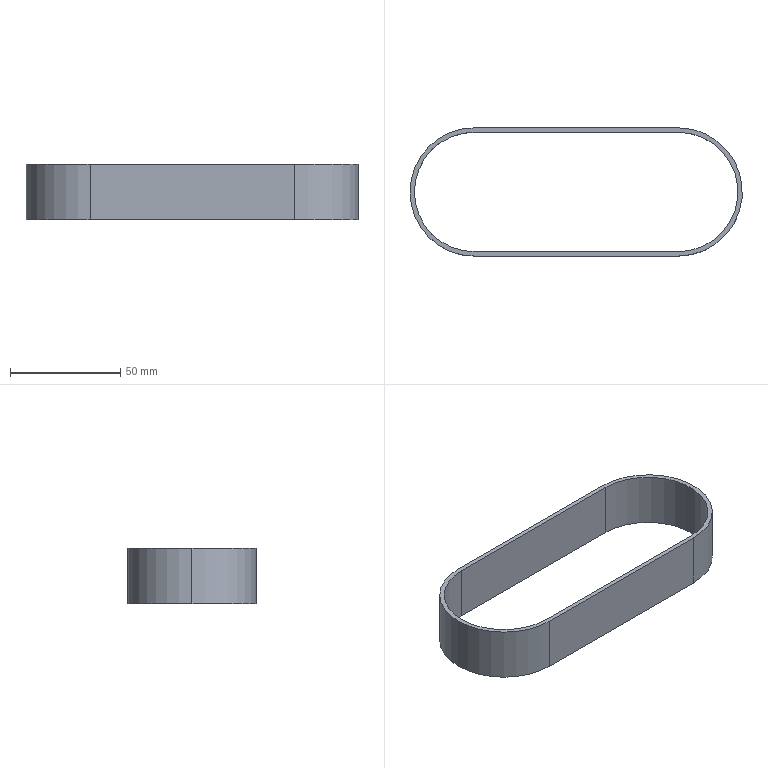Part | STEP file | HTBNV355-S5M-250 high-torque timing belt S5M MISUMI 24 | 1 solid | 12 faces | box 150.61 x 58.11 x 25 mm | volume 18064 mm3 | cylinder 6 | plane 6 | commonest cylinder face diameters 54.11 x3 58.11 x3
STEP:
#1=CARTESIAN_POINT('',(-46.25,27.055,12.5));
#2=VERTEX_POINT('',#1);
#3=CARTESIAN_POINT('',(-73.305,0.,12.5));
#4=VERTEX_POINT('',#3);
#5=CARTESIAN_POINT('',(-46.25,0.,12.5));
#6=DIRECTION('',(0.,0.,1.));
#7=DIRECTION('',(1.,0.,0.));
#8=AXIS2_PLACEMENT_3D('',#5,#6,#7);
#9=CIRCLE('',#8,27.055);
#10=EDGE_CURVE('',#2,#4,#9,.T.);
#11=ORIENTED_EDGE('',*,*,#10,.T.);
#12=CARTESIAN_POINT('',(-73.305,0.,-12.5));
#13=VERTEX_POINT('',#12);
#14=CARTESIAN_POINT('',(-73.305,0.,12.5));
#15=DIRECTION('',(0.,0.,-1.));
#16=VECTOR('',#15,1000.);
#17=LINE('',#14,#16);
#18=EDGE_CURVE('',#4,#13,#17,.T.);
#19=ORIENTED_EDGE('',*,*,#18,.T.);
#20=CARTESIAN_POINT('',(-46.25,27.055,-12.5));
#21=VERTEX_POINT('',#20);
#22=CARTESIAN_POINT('',(-46.25,0.,-12.5));
#23=DIRECTION('',(0.,0.,1.));
#24=DIRECTION('',(1.,0.,0.));
#25=AXIS2_PLACEMENT_3D('',#22,#23,#24);
#26=CIRCLE('',#25,27.055);
#27=EDGE_CURVE('',#21,#13,#26,.T.);
#28=ORIENTED_EDGE('',*,*,#27,.F.);
#29=CARTESIAN_POINT('',(-46.25,27.055,12.5));
#30=DIRECTION('',(0.,0.,-1.));
#31=VECTOR('',#30,1000.);
#32=LINE('',#29,#31);
#33=EDGE_CURVE('',#2,#21,#32,.T.);
#34=ORIENTED_EDGE('',*,*,#33,.F.);
#35=EDGE_LOOP('',(#11,#19,#28,#34));
#36=FACE_OUTER_BOUND('',#35,.T.);
#37=CARTESIAN_POINT('',(-46.25,0.,12.5));
#38=DIRECTION('',(0.,0.,-1.));
#39=DIRECTION('',(-1.,0.,0.));
#40=AXIS2_PLACEMENT_3D('',#37,#38,#39);
#41=CYLINDRICAL_SURFACE('',#40,27.055);
#42=ADVANCED_FACE('',(#36),#41,.F.);
#43=CARTESIAN_POINT('',(-75.305,0.,12.5));
#44=VERTEX_POINT('',#43);
#45=CARTESIAN_POINT('',(-46.25,-29.055,12.5));
#46=VERTEX_POINT('',#45);
#47=CARTESIAN_POINT('',(-46.25,0.,12.5));
#48=DIRECTION('',(0.,0.,1.));
#49=DIRECTION('',(1.,0.,0.));
#50=AXIS2_PLACEMENT_3D('',#47,#48,#49);
#51=CIRCLE('',#50,29.055);
#52=EDGE_CURVE('',#44,#46,#51,.T.);
#53=ORIENTED_EDGE('',*,*,#52,.F.);
#54=CARTESIAN_POINT('',(-75.305,0.,-12.5));
#55=VERTEX_POINT('',#54);
#56=CARTESIAN_POINT('',(-75.305,0.,12.5));
#57=DIRECTION('',(0.,0.,-1.));
#58=VECTOR('',#57,1000.);
#59=LINE('',#56,#58);
#60=EDGE_CURVE('',#44,#55,#59,.T.);
#61=ORIENTED_EDGE('',*,*,#60,.T.);
#62=CARTESIAN_POINT('',(-46.25,-29.055,-12.5));
#63=VERTEX_POINT('',#62);
#64=CARTESIAN_POINT('',(-46.25,0.,-12.5));
#65=DIRECTION('',(0.,0.,1.));
#66=DIRECTION('',(1.,0.,0.));
#67=AXIS2_PLACEMENT_3D('',#64,#65,#66);
#68=CIRCLE('',#67,29.055);
#69=EDGE_CURVE('',#55,#63,#68,.T.);
#70=ORIENTED_EDGE('',*,*,#69,.T.);
#71=CARTESIAN_POINT('',(-46.25,-29.055,12.5));
#72=DIRECTION('',(0.,0.,-1.));
#73=VECTOR('',#72,1000.);
#74=LINE('',#71,#73);
#75=EDGE_CURVE('',#46,#63,#74,.T.);
#76=ORIENTED_EDGE('',*,*,#75,.F.);
#77=EDGE_LOOP('',(#53,#61,#70,#76));
#78=FACE_OUTER_BOUND('',#77,.T.);
#79=CARTESIAN_POINT('',(-46.25,0.,12.5));
#80=DIRECTION('',(0.,0.,-1.));
#81=DIRECTION('',(-1.,0.,0.));
#82=AXIS2_PLACEMENT_3D('',#79,#80,#81);
#83=CYLINDRICAL_SURFACE('',#82,29.055);
#84=ADVANCED_FACE('',(#78),#83,.T.);
#85=CARTESIAN_POINT('',(-46.25,29.055,12.5));
#86=VERTEX_POINT('',#85);
#87=CARTESIAN_POINT('',(-46.25,0.,12.5));
#88=DIRECTION('',(0.,0.,1.));
#89=DIRECTION('',(1.,0.,0.));
#90=AXIS2_PLACEMENT_3D('',#87,#88,#89);
#91=CIRCLE('',#90,29.055);
#92=EDGE_CURVE('',#86,#44,#91,.T.);
#93=ORIENTED_EDGE('',*,*,#92,.T.);
#94=ORIENTED_EDGE('',*,*,#52,.T.);
#95=CARTESIAN_POINT('',(46.25,-29.055,12.5));
#96=VERTEX_POINT('',#95);
#97=CARTESIAN_POINT('',(-46.25,-29.055,12.5));
#98=DIRECTION('',(1.,0.,0.));
#99=VECTOR('',#98,1000.);
#100=LINE('',#97,#99);
#101=EDGE_CURVE('',#46,#96,#100,.T.);
#102=ORIENTED_EDGE('',*,*,#101,.T.);
#103=CARTESIAN_POINT('',(46.25,29.055,12.5));
#104=VERTEX_POINT('',#103);
#105=CARTESIAN_POINT('',(46.25,0.,12.5));
#106=DIRECTION('',(0.,0.,1.));
#107=DIRECTION('',(1.,0.,0.));
#108=AXIS2_PLACEMENT_3D('',#105,#106,#107);
#109=CIRCLE('',#108,29.055);
#110=EDGE_CURVE('',#96,#104,#109,.T.);
#111=ORIENTED_EDGE('',*,*,#110,.T.);
#112=CARTESIAN_POINT('',(-46.25,29.055,12.5));
#113=DIRECTION('',(-1.,0.,0.));
#114=VECTOR('',#113,1000.);
#115=LINE('',#112,#114);
#116=EDGE_CURVE('',#104,#86,#115,.T.);
#117=ORIENTED_EDGE('',*,*,#116,.T.);
#118=EDGE_LOOP('',(#93,#94,#102,#111,#117));
#119=FACE_OUTER_BOUND('',#118,.T.);
#120=CARTESIAN_POINT('',(-46.25,-27.055,12.5));
#121=VERTEX_POINT('',#120);
#122=CARTESIAN_POINT('',(46.25,-27.055,12.5));
#123=VERTEX_POINT('',#122);
#124=CARTESIAN_POINT('',(-46.25,-27.055,12.5));
#125=DIRECTION('',(1.,0.,0.));
#126=VECTOR('',#125,1000.);
#127=LINE('',#124,#126);
#128=EDGE_CURVE('',#121,#123,#127,.T.);
#129=ORIENTED_EDGE('',*,*,#128,.F.);
#130=CARTESIAN_POINT('',(-46.25,0.,12.5));
#131=DIRECTION('',(0.,0.,1.));
#132=DIRECTION('',(1.,0.,0.));
#133=AXIS2_PLACEMENT_3D('',#130,#131,#132);
#134=CIRCLE('',#133,27.055);
#135=EDGE_CURVE('',#4,#121,#134,.T.);
#136=ORIENTED_EDGE('',*,*,#135,.F.);
#137=ORIENTED_EDGE('',*,*,#10,.F.);
#138=CARTESIAN_POINT('',(46.25,27.055,12.5));
#139=VERTEX_POINT('',#138);
#140=CARTESIAN_POINT('',(-46.25,27.055,12.5));
#141=DIRECTION('',(-1.,0.,0.));
#142=VECTOR('',#141,1000.);
#143=LINE('',#140,#142);
#144=EDGE_CURVE('',#139,#2,#143,.T.);
#145=ORIENTED_EDGE('',*,*,#144,.F.);
#146=CARTESIAN_POINT('',(46.25,0.,12.5));
#147=DIRECTION('',(0.,0.,1.));
#148=DIRECTION('',(1.,0.,0.));
#149=AXIS2_PLACEMENT_3D('',#146,#147,#148);
#150=CIRCLE('',#149,27.055);
#151=EDGE_CURVE('',#123,#139,#150,.T.);
#152=ORIENTED_EDGE('',*,*,#151,.F.);
#153=EDGE_LOOP('',(#129,#136,#137,#145,#152));
#154=FACE_BOUND('',#153,.T.);
#155=CARTESIAN_POINT('',(-46.25,0.,12.5));
#156=DIRECTION('',(0.,0.,1.));
#157=DIRECTION('',(1.,0.,0.));
#158=AXIS2_PLACEMENT_3D('',#155,#156,#157);
#159=PLANE('',#158);
#160=ADVANCED_FACE('',(#119,#154),#159,.T.);
#161=CARTESIAN_POINT('',(-46.25,29.055,-12.5));
#162=VERTEX_POINT('',#161);
#163=CARTESIAN_POINT('',(-46.25,0.,-12.5));
#164=DIRECTION('',(0.,0.,1.));
#165=DIRECTION('',(1.,0.,0.));
#166=AXIS2_PLACEMENT_3D('',#163,#164,#165);
#167=CIRCLE('',#166,29.055);
#168=EDGE_CURVE('',#162,#55,#167,.T.);
#169=ORIENTED_EDGE('',*,*,#168,.F.);
#170=CARTESIAN_POINT('',(46.25,29.055,-12.5));
#171=VERTEX_POINT('',#170);
#172=CARTESIAN_POINT('',(-46.25,29.055,-12.5));
#173=DIRECTION('',(-1.,0.,0.));
#174=VECTOR('',#173,1000.);
#175=LINE('',#172,#174);
#176=EDGE_CURVE('',#171,#162,#175,.T.);
#177=ORIENTED_EDGE('',*,*,#176,.F.);
#178=CARTESIAN_POINT('',(46.25,-29.055,-12.5));
#179=VERTEX_POINT('',#178);
#180=CARTESIAN_POINT('',(46.25,0.,-12.5));
#181=DIRECTION('',(0.,0.,1.));
#182=DIRECTION('',(1.,0.,0.));
#183=AXIS2_PLACEMENT_3D('',#180,#181,#182);
#184=CIRCLE('',#183,29.055);
#185=EDGE_CURVE('',#179,#171,#184,.T.);
#186=ORIENTED_EDGE('',*,*,#185,.F.);
#187=CARTESIAN_POINT('',(-46.25,-29.055,-12.5));
#188=DIRECTION('',(1.,0.,0.));
#189=VECTOR('',#188,1000.);
#190=LINE('',#187,#189);
#191=EDGE_CURVE('',#63,#179,#190,.T.);
#192=ORIENTED_EDGE('',*,*,#191,.F.);
#193=ORIENTED_EDGE('',*,*,#69,.F.);
#194=EDGE_LOOP('',(#169,#177,#186,#192,#193));
#195=FACE_OUTER_BOUND('',#194,.T.);
#196=ORIENTED_EDGE('',*,*,#27,.T.);
#197=CARTESIAN_POINT('',(-46.25,-27.055,-12.5));
#198=VERTEX_POINT('',#197);
#199=CARTESIAN_POINT('',(-46.25,0.,-12.5));
#200=DIRECTION('',(0.,0.,1.));
#201=DIRECTION('',(1.,0.,0.));
#202=AXIS2_PLACEMENT_3D('',#199,#200,#201);
#203=CIRCLE('',#202,27.055);
#204=EDGE_CURVE('',#13,#198,#203,.T.);
#205=ORIENTED_EDGE('',*,*,#204,.T.);
#206=CARTESIAN_POINT('',(46.25,-27.055,-12.5));
#207=VERTEX_POINT('',#206);
#208=CARTESIAN_POINT('',(-46.25,-27.055,-12.5));
#209=DIRECTION('',(1.,0.,0.));
#210=VECTOR('',#209,1000.);
#211=LINE('',#208,#210);
#212=EDGE_CURVE('',#198,#207,#211,.T.);
#213=ORIENTED_EDGE('',*,*,#212,.T.);
#214=CARTESIAN_POINT('',(46.25,27.055,-12.5));
#215=VERTEX_POINT('',#214);
#216=CARTESIAN_POINT('',(46.25,0.,-12.5));
#217=DIRECTION('',(0.,0.,1.));
#218=DIRECTION('',(1.,0.,0.));
#219=AXIS2_PLACEMENT_3D('',#216,#217,#218);
#220=CIRCLE('',#219,27.055);
#221=EDGE_CURVE('',#207,#215,#220,.T.);
#222=ORIENTED_EDGE('',*,*,#221,.T.);
#223=CARTESIAN_POINT('',(-46.25,27.055,-12.5));
#224=DIRECTION('',(-1.,0.,0.));
#225=VECTOR('',#224,1000.);
#226=LINE('',#223,#225);
#227=EDGE_CURVE('',#215,#21,#226,.T.);
#228=ORIENTED_EDGE('',*,*,#227,.T.);
#229=EDGE_LOOP('',(#196,#205,#213,#222,#228));
#230=FACE_BOUND('',#229,.T.);
#231=CARTESIAN_POINT('',(-46.25,0.,-12.5));
#232=DIRECTION('',(0.,0.,1.));
#233=DIRECTION('',(1.,0.,0.));
#234=AXIS2_PLACEMENT_3D('',#231,#232,#233);
#235=PLANE('',#234);
#236=ADVANCED_FACE('',(#195,#230),#235,.F.);
#237=ORIENTED_EDGE('',*,*,#60,.F.);
#238=ORIENTED_EDGE('',*,*,#92,.F.);
#239=CARTESIAN_POINT('',(-46.25,29.055,12.5));
#240=DIRECTION('',(0.,0.,-1.));
#241=VECTOR('',#240,1000.);
#242=LINE('',#239,#241);
#243=EDGE_CURVE('',#86,#162,#242,.T.);
#244=ORIENTED_EDGE('',*,*,#243,.T.);
#245=ORIENTED_EDGE('',*,*,#168,.T.);
#246=EDGE_LOOP('',(#237,#238,#244,#245));
#247=FACE_OUTER_BOUND('',#246,.T.);
#248=CARTESIAN_POINT('',(-46.25,0.,12.5));
#249=DIRECTION('',(0.,0.,-1.));
#250=DIRECTION('',(-1.,0.,0.));
#251=AXIS2_PLACEMENT_3D('',#248,#249,#250);
#252=CYLINDRICAL_SURFACE('',#251,29.055);
#253=ADVANCED_FACE('',(#247),#252,.T.);
#254=ORIENTED_EDGE('',*,*,#191,.T.);
#255=CARTESIAN_POINT('',(46.25,-29.055,12.5));
#256=DIRECTION('',(0.,0.,-1.));
#257=VECTOR('',#256,1000.);
#258=LINE('',#255,#257);
#259=EDGE_CURVE('',#96,#179,#258,.T.);
#260=ORIENTED_EDGE('',*,*,#259,.F.);
#261=ORIENTED_EDGE('',*,*,#101,.F.);
#262=ORIENTED_EDGE('',*,*,#75,.T.);
#263=EDGE_LOOP('',(#254,#260,#261,#262));
#264=FACE_OUTER_BOUND('',#263,.T.);
#265=CARTESIAN_POINT('',(-46.25,-29.055,12.5));
#266=DIRECTION('',(0.,1.,0.));
#267=DIRECTION('',(-1.,0.,0.));
#268=AXIS2_PLACEMENT_3D('',#265,#266,#267);
#269=PLANE('',#268);
#270=ADVANCED_FACE('',(#264),#269,.F.);
#271=ORIENTED_EDGE('',*,*,#185,.T.);
#272=CARTESIAN_POINT('',(46.25,29.055,12.5));
#273=DIRECTION('',(0.,0.,-1.));
#274=VECTOR('',#273,1000.);
#275=LINE('',#272,#274);
#276=EDGE_CURVE('',#104,#171,#275,.T.);
#277=ORIENTED_EDGE('',*,*,#276,.F.);
#278=ORIENTED_EDGE('',*,*,#110,.F.);
#279=ORIENTED_EDGE('',*,*,#259,.T.);
#280=EDGE_LOOP('',(#271,#277,#278,#279));
#281=FACE_OUTER_BOUND('',#280,.T.);
#282=CARTESIAN_POINT('',(46.25,0.,12.5));
#283=DIRECTION('',(0.,0.,-1.));
#284=DIRECTION('',(-1.,0.,0.));
#285=AXIS2_PLACEMENT_3D('',#282,#283,#284);
#286=CYLINDRICAL_SURFACE('',#285,29.055);
#287=ADVANCED_FACE('',(#281),#286,.T.);
#288=ORIENTED_EDGE('',*,*,#176,.T.);
#289=ORIENTED_EDGE('',*,*,#243,.F.);
#290=ORIENTED_EDGE('',*,*,#116,.F.);
#291=ORIENTED_EDGE('',*,*,#276,.T.);
#292=EDGE_LOOP('',(#288,#289,#290,#291));
#293=FACE_OUTER_BOUND('',#292,.T.);
#294=CARTESIAN_POINT('',(-46.25,29.055,12.5));
#295=DIRECTION('',(0.,-1.,0.));
#296=DIRECTION('',(1.,0.,0.));
#297=AXIS2_PLACEMENT_3D('',#294,#295,#296);
#298=PLANE('',#297);
#299=ADVANCED_FACE('',(#293),#298,.F.);
#300=ORIENTED_EDGE('',*,*,#18,.F.);
#301=ORIENTED_EDGE('',*,*,#135,.T.);
#302=CARTESIAN_POINT('',(-46.25,-27.055,12.5));
#303=DIRECTION('',(0.,0.,-1.));
#304=VECTOR('',#303,1000.);
#305=LINE('',#302,#304);
#306=EDGE_CURVE('',#121,#198,#305,.T.);
#307=ORIENTED_EDGE('',*,*,#306,.T.);
#308=ORIENTED_EDGE('',*,*,#204,.F.);
#309=EDGE_LOOP('',(#300,#301,#307,#308));
#310=FACE_OUTER_BOUND('',#309,.T.);
#311=CARTESIAN_POINT('',(-46.25,0.,12.5));
#312=DIRECTION('',(0.,0.,-1.));
#313=DIRECTION('',(-1.,0.,0.));
#314=AXIS2_PLACEMENT_3D('',#311,#312,#313);
#315=CYLINDRICAL_SURFACE('',#314,27.055);
#316=ADVANCED_FACE('',(#310),#315,.F.);
#317=ORIENTED_EDGE('',*,*,#212,.F.);
#318=ORIENTED_EDGE('',*,*,#306,.F.);
#319=ORIENTED_EDGE('',*,*,#128,.T.);
#320=CARTESIAN_POINT('',(46.25,-27.055,12.5));
#321=DIRECTION('',(0.,0.,-1.));
#322=VECTOR('',#321,1000.);
#323=LINE('',#320,#322);
#324=EDGE_CURVE('',#123,#207,#323,.T.);
#325=ORIENTED_EDGE('',*,*,#324,.T.);
#326=EDGE_LOOP('',(#317,#318,#319,#325));
#327=FACE_OUTER_BOUND('',#326,.T.);
#328=CARTESIAN_POINT('',(-46.25,-27.055,12.5));
#329=DIRECTION('',(0.,1.,0.));
#330=DIRECTION('',(0.,0.,1.));
#331=AXIS2_PLACEMENT_3D('',#328,#329,#330);
#332=PLANE('',#331);
#333=ADVANCED_FACE('',(#327),#332,.T.);
#334=ORIENTED_EDGE('',*,*,#221,.F.);
#335=ORIENTED_EDGE('',*,*,#324,.F.);
#336=ORIENTED_EDGE('',*,*,#151,.T.);
#337=CARTESIAN_POINT('',(46.25,27.055,12.5));
#338=DIRECTION('',(0.,0.,-1.));
#339=VECTOR('',#338,1000.);
#340=LINE('',#337,#339);
#341=EDGE_CURVE('',#139,#215,#340,.T.);
#342=ORIENTED_EDGE('',*,*,#341,.T.);
#343=EDGE_LOOP('',(#334,#335,#336,#342));
#344=FACE_OUTER_BOUND('',#343,.T.);
#345=CARTESIAN_POINT('',(46.25,0.,12.5));
#346=DIRECTION('',(0.,0.,-1.));
#347=DIRECTION('',(-1.,0.,0.));
#348=AXIS2_PLACEMENT_3D('',#345,#346,#347);
#349=CYLINDRICAL_SURFACE('',#348,27.055);
#350=ADVANCED_FACE('',(#344),#349,.F.);
#351=ORIENTED_EDGE('',*,*,#227,.F.);
#352=ORIENTED_EDGE('',*,*,#341,.F.);
#353=ORIENTED_EDGE('',*,*,#144,.T.);
#354=ORIENTED_EDGE('',*,*,#33,.T.);
#355=EDGE_LOOP('',(#351,#352,#353,#354));
#356=FACE_OUTER_BOUND('',#355,.T.);
#357=CARTESIAN_POINT('',(-46.25,27.055,12.5));
#358=DIRECTION('',(0.,-1.,0.));
#359=DIRECTION('',(1.,0.,0.));
#360=AXIS2_PLACEMENT_3D('',#357,#358,#359);
#361=PLANE('',#360);
#362=ADVANCED_FACE('',(#356),#361,.T.);
#363=CLOSED_SHELL('',(#42,#84,#160,#236,#253,#270,#287,#299,#316,#333,#350,#362));
#364=MANIFOLD_SOLID_BREP('',#363);
#365=CARTESIAN_POINT('',(0.,0.,0.));
#366=DIRECTION('',(0.,0.,1.));
#367=DIRECTION('',(1.,0.,0.));
#368=AXIS2_PLACEMENT_3D('',#365,#366,#367);
#369=(LENGTH_UNIT()NAMED_UNIT(*)SI_UNIT(.MILLI.,.METRE.));
#370=UNCERTAINTY_MEASURE_WITH_UNIT(LENGTH_MEASURE(0.00001),#369,'','');
#371=(NAMED_UNIT(*)PLANE_ANGLE_UNIT()SI_UNIT($,.RADIAN.));
#372=(NAMED_UNIT(*)SI_UNIT($,.STERADIAN.)SOLID_ANGLE_UNIT());
#373=(GEOMETRIC_REPRESENTATION_CONTEXT(3)GLOBAL_UNCERTAINTY_ASSIGNED_CONTEXT((#370))GLOBAL_UNIT_ASSIGNED_CONTEXT((#369,#371,#372))REPRESENTATION_CONTEXT('',''));
#374=ADVANCED_BREP_SHAPE_REPRESENTATION('',(#364,#368),#373);